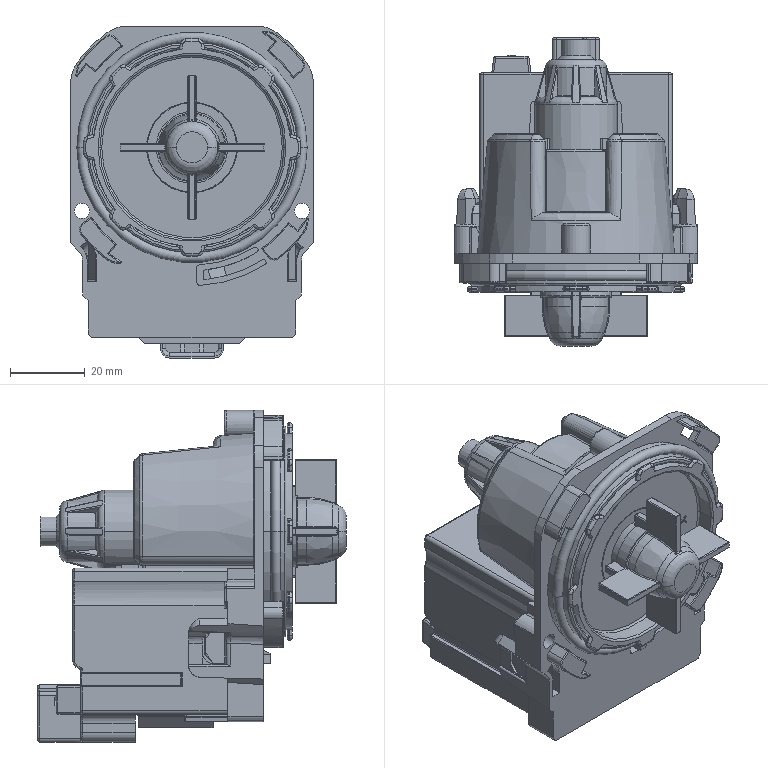Part | STEP file | ZXW735-L-25 | 1 solid | 2836 faces | box 65 x 82.55 x 88.85 mm | volume 144092 mm3 | plane 1166 | cylinder 894 | torus 373 | spline 195 | cone 131 | sphere 76 | other 1 | commonest cylinder face diameters 0.6 x206 1 x132 2 x116 0.4 x102 12.566 x36 3 x26